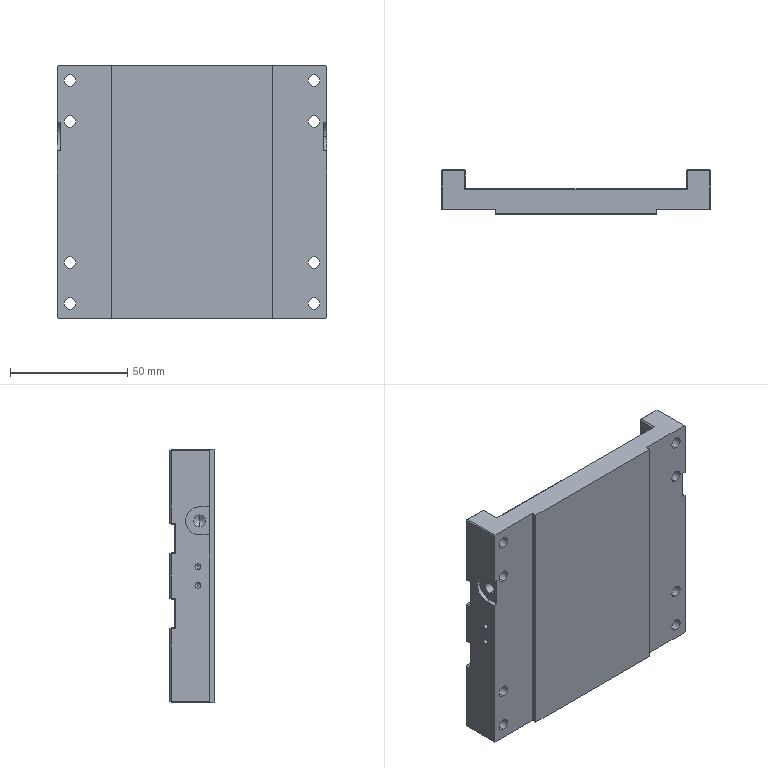Part | STEP file | LES120 slide base^FTH120-PD-direct-drive motor | 1 solid | 163 faces | box 115 x 18.873 x 108 mm | volume 136774 mm3 | plane 116 | cylinder 35 | cone 12 | commonest cylinder face diameters 5 x20 2.5 x8 6 x4 12 x3